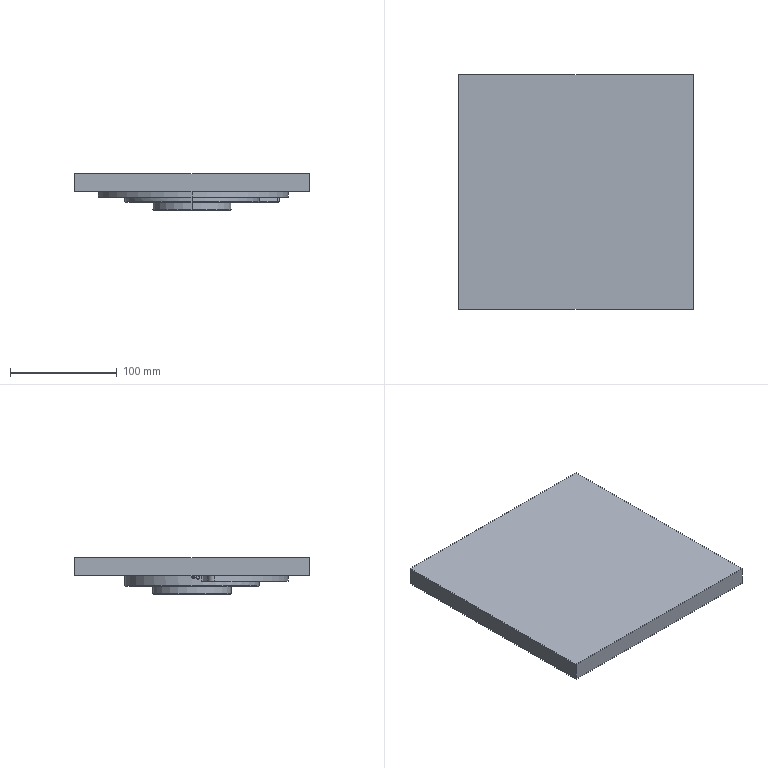NC program | NX | posted with a generic post | part box 220 x 220 x 34.5 mm
Lines 4490 to 5339 of 14163:
(ZLEVEL_PROFILE_COPY_1_COPY , TOOL : D4)
N8918 T10 M6
N8920 G54
N8922 G17 G0 G90 X68.105 Y9.166 S9500 M3
N8924 G43 Z30. H10
N8926 Z-0.4
N8928 G94 G1 X67.66 Y9.696 F1000.
N8930 G3 X67.284 Y9.833 R0.4
N8932 G1 X64.343 Y9.315 F1500.
N8934 X64.337 Y9.257
N8936 G2 X64.684 Y6.399 R65.
N8938 G3 X64.917 Y6.074 R0.4
N8940 G1 X65.545 Y5.79
N8942 G0 X68.105 Y9.166 Z-0.8
N8944 G1 X67.66 Y9.696 F1000.
N8946 G3 X67.284 Y9.833 R0.4
N8948 G1 X64.343 Y9.315 F1500.
N8950 X64.337 Y9.257
N8952 G2 X64.684 Y6.398 R65.
N8954 G3 X64.917 Y6.073 R0.4
N8956 G1 X65.545 Y5.789
N8958 G0 X68.105 Y9.166 Z-1.2
N8960 G1 X67.66 Y9.696 F1000.
N8962 G3 X67.284 Y9.833 R0.4
N8964 G1 X64.343 Y9.315 F1500.
N8966 X64.337 Y9.257
N8968 G2 X64.684 Y6.397 R65.
N8970 G3 X64.918 Y6.072 R0.4
N8972 G1 X65.545 Y5.788
N8974 G0 X68.105 Y9.166 Z-1.6
N8976 G1 X67.66 Y9.696 F1000.
N8978 G3 X67.284 Y9.833 R0.4
N8980 G1 X64.343 Y9.315 F1500.
N8982 X64.338 Y9.257
N8984 G2 X64.685 Y6.396 R65.
N8986 G3 X64.918 Y6.071 R0.4
N8988 G1 X65.545 Y5.787
N8990 G0 X68.105 Y9.166 Z-2.
N8992 G1 X67.66 Y9.696 F1000.
N8994 G3 X67.284 Y9.833 R0.4
N8996 G1 X64.343 Y9.315 F1500.
N8998 X64.338 Y9.257
N9000 G2 X64.685 Y6.395 R65.
N9002 G3 X64.918 Y6.069 R0.4
N9004 G1 X65.545 Y5.786
N9006 G0 X68.105 Y9.166 Z-2.4
N9008 G1 X67.66 Y9.696 F1000.
N9010 G3 X67.284 Y9.833 R0.4
N9012 G1 X64.343 Y9.315 F1500.
N9014 X64.338 Y9.256
N9016 G2 X64.685 Y6.393 R65.
N9018 G3 X64.918 Y6.068 R0.4
N9020 G1 X65.545 Y5.784
N9022 G0 X68.105 Y9.166 Z-2.8
N9024 G1 X67.66 Y9.696 F1000.
N9026 G3 X67.284 Y9.833 R0.4
N9028 G1 X64.343 Y9.315 F1500.
N9030 X64.338 Y9.256
N9032 G2 X64.686 Y6.386 R65.
N9034 G3 X64.919 Y6.061 R0.4
N9036 G1 X65.546 Y5.777
N9038 G0 X68.105 Y9.166 Z-3.2
N9040 G1 X67.66 Y9.696 F1000.
N9042 G3 X67.284 Y9.833 R0.4
N9044 G1 X64.343 Y9.315 F1500.
N9046 X64.338 Y9.256
N9048 G2 X64.686 Y6.386 R65.
N9050 G3 X64.919 Y6.061 R0.4
N9052 G1 X65.546 Y5.777
N9054 G0 X68.105 Y9.166 Z-3.6
N9056 G1 X67.66 Y9.696 F1000.
N9058 G3 X67.284 Y9.833 R0.4
N9060 G1 X64.343 Y9.315 F1500.
N9062 X64.338 Y9.256
N9064 G2 X64.686 Y6.386 R65.
N9066 G3 X64.919 Y6.061 R0.4
N9068 G1 X65.546 Y5.777
N9070 G0 X68.105 Y9.166 Z-4.
N9072 G1 X67.66 Y9.696 F1000.
N9074 G3 X67.284 Y9.833 R0.4
N9076 G1 X64.343 Y9.315 F1500.
N9078 X64.338 Y9.256
N9080 G2 X64.686 Y6.386 R65.
N9082 G3 X64.919 Y6.061 R0.4
N9084 G1 X65.546 Y5.777
N9086 G0 X68.105 Y9.166 Z-4.4
N9088 G1 X67.66 Y9.696 F1000.
N9090 G3 X67.284 Y9.833 R0.4
N9092 G1 X64.343 Y9.315 F1500.
N9094 X64.338 Y9.256
N9096 G2 X64.686 Y6.386 R65.
N9098 G3 X64.919 Y6.061 R0.4
N9100 G1 X65.546 Y5.777
N9102 G0 X68.105 Y9.166 Z-4.8
N9104 G1 X67.66 Y9.696 F1000.
N9106 G3 X67.284 Y9.833 R0.4
N9108 G1 X64.343 Y9.315 F1500.
N9110 X64.338 Y9.256
N9112 G2 X64.686 Y6.386 R65.
N9114 G3 X64.919 Y6.061 R0.4
N9116 G1 X65.546 Y5.777
N9118 G0 X68.105 Y9.166 Z-5.2
N9120 G1 X67.66 Y9.696 F1000.
N9122 G3 X67.284 Y9.833 R0.4
N9124 G1 X64.343 Y9.315 F1500.
N9126 X64.338 Y9.256
N9128 G2 X64.686 Y6.386 R65.
N9130 G3 X64.919 Y6.061 R0.4
N9132 G1 X65.546 Y5.777
N9134 G0 X68.105 Y9.166 Z-5.6
N9136 G1 X67.66 Y9.696 F1000.
N9138 G3 X67.284 Y9.833 R0.4
N9140 G1 X64.343 Y9.315 F1500.
N9142 X64.338 Y9.256
N9144 G2 X64.686 Y6.386 R65.
N9146 G3 X64.919 Y6.061 R0.4
N9148 G1 X65.546 Y5.777
N9150 G0 X68.105 Y9.166 Z-6.
N9152 G1 X67.66 Y9.696 F1000.
N9154 G3 X67.284 Y9.833 R0.4
N9156 G1 X64.343 Y9.315 F1500.
N9158 X64.338 Y9.256
N9160 G2 X64.686 Y6.386 R65.
N9162 G3 X64.919 Y6.061 R0.4
N9164 G1 X65.546 Y5.777
N9166 G0 X68.105 Y9.166 Z-6.4
N9168 G1 X67.66 Y9.696 F1000.
N9170 G3 X67.284 Y9.833 R0.4
N9172 G1 X64.343 Y9.315 F1500.
N9174 X64.338 Y9.256
N9176 G2 X64.686 Y6.386 R65.
N9178 G3 X64.919 Y6.061 R0.4
N9180 G1 X65.546 Y5.777
N9182 G0 X68.105 Y9.166 Z-6.8
N9184 G1 X67.66 Y9.696 F1000.
N9186 G3 X67.284 Y9.833 R0.4
N9188 G1 X64.343 Y9.315 F1500.
N9190 X64.338 Y9.256
N9192 G2 X64.685 Y6.388 R65.
N9194 G3 X64.918 Y6.062 R0.4
N9196 G1 X65.545 Y5.779
N9198 G0 X68.105 Y9.166 Z-7.2
N9200 G1 X67.659 Y9.696 F1000.
N9202 G3 X67.284 Y9.833 R0.4
N9204 G1 X64.343 Y9.315 F1500.
N9206 X64.338 Y9.255
N9208 G2 X64.523 Y7.856 R65.
N9210 G1 X64.651 Y6.699
N9212 G3 X64.888 Y6.377 R0.4
N9214 G1 X65.517 Y6.101
N9216 G0 X68.105 Y9.166 Z-7.6
N9218 G1 X67.66 Y9.696 F1000.
N9220 G3 X67.284 Y9.833 R0.4
N9222 G1 X64.343 Y9.315 F1500.
N9224 X64.338 Y9.255
N9226 G2 X64.523 Y7.856 R65.
N9228 G1 X64.522 Y7.838
N9230 X64.598 Y7.19
N9232 X64.613 Y7.053
N9234 X64.651 Y6.699
N9236 G3 X64.886 Y6.376 R0.4
N9238 G1 X65.517 Y6.096
N9240 G0 X68.105 Y9.166 Z-8.
N9242 G1 X67.66 Y9.696 F1000.
N9244 G3 X67.284 Y9.833 R0.4
N9246 G1 X64.343 Y9.315 F1500.
N9248 X64.338 Y9.255
N9250 G2 X64.523 Y7.856 R65.
N9252 G1 X64.522 Y7.838
N9254 X64.599 Y7.19
N9256 X64.613 Y7.053
N9258 X64.651 Y6.699
N9260 G3 X64.886 Y6.376 R0.4
N9262 G1 X65.517 Y6.096
N9264 G0 X68.105 Y9.166 Z-8.4
N9266 G1 X67.66 Y9.696 F1000.
N9268 G3 X67.284 Y9.833 R0.4
N9270 G1 X64.343 Y9.315 F1500.
N9272 X64.338 Y9.255
N9274 G2 X64.523 Y7.856 R65.
N9276 G1 X64.522 Y7.838
N9278 X64.599 Y7.19
N9280 X64.613 Y7.053
N9282 X64.651 Y6.699
N9284 G3 X64.886 Y6.376 R0.4
N9286 G1 X65.517 Y6.096
N9288 G0 X68.105 Y9.166 Z-8.8
N9290 G1 X67.66 Y9.696 F1000.
N9292 G3 X67.284 Y9.833 R0.4
N9294 G1 X64.343 Y9.315 F1500.
N9296 X64.338 Y9.255
N9298 G2 X64.523 Y7.856 R65.
N9300 G1 X64.522 Y7.838
N9302 X64.613 Y7.062
N9304 X64.651 Y6.699
N9306 G3 X64.887 Y6.376 R0.4
N9308 G1 X65.517 Y6.097
N9310 G0 X68.106 Y9.166 Z-9.2
N9312 G1 X67.66 Y9.696 F1000.
N9314 G3 X67.284 Y9.833 R0.4
N9316 G1 X64.343 Y9.315 F1500.
N9318 X64.338 Y9.255
N9320 G2 X64.523 Y7.856 R65.
N9322 G1 X64.629 Y6.908
N9324 X64.651 Y6.699
N9326 G3 X64.885 Y6.375 R0.4
N9328 G1 X65.518 Y6.089
N9330 G0 X68.106 Y9.166 Z-9.6
N9332 G1 X67.66 Y9.696 F1000.
N9334 G3 X67.284 Y9.833 R0.4
N9336 G1 X64.343 Y9.315 F1500.
N9338 X64.338 Y9.255
N9340 G2 X64.523 Y7.856 R65.
N9342 G3 X64.764 Y7.537 R0.4
N9344 G1 X65.391 Y7.269
N9346 G0 X68.106 Y9.166 Z-10.
N9348 G1 X67.66 Y9.696 F1000.
N9350 G3 X67.285 Y9.833 R0.4
N9352 G1 X64.343 Y9.315 F1500.
N9354 X64.338 Y9.255
N9356 G2 X64.523 Y7.856 R65.
N9358 G3 X64.764 Y7.537 R0.4
N9360 G1 X65.391 Y7.27
N9362 G0 X68.106 Y9.166 Z-10.4
N9364 G1 X67.66 Y9.696 F1000.
N9366 G3 X67.285 Y9.833 R0.4
N9368 G1 X64.343 Y9.315 F1500.
N9370 X64.338 Y9.255
N9372 G2 X64.523 Y7.856 R65.
N9374 G3 X64.764 Y7.537 R0.4
N9376 G1 X65.391 Y7.269
N9378 G0 X68.106 Y9.166 Z-10.8
N9380 G1 X67.66 Y9.696 F1000.
N9382 G3 X67.285 Y9.833 R0.4
N9384 G1 X64.343 Y9.315 F1500.
N9386 X64.338 Y9.255
N9388 G2 X64.523 Y7.856 R65.
N9390 G3 X64.764 Y7.537 R0.4
N9392 G1 X65.391 Y7.269
N9394 G0 X68.106 Y9.166 Z-11.2
N9396 G1 X67.66 Y9.696 F1000.
N9398 G3 X67.285 Y9.833 R0.4
N9400 G1 X64.343 Y9.315 F1500.
N9402 X64.338 Y9.255
N9404 G2 X64.523 Y7.856 R65.
N9406 G3 X64.764 Y7.537 R0.4
N9408 G1 X65.391 Y7.269
N9410 G0 X68.106 Y9.166 Z-11.6
N9412 G1 X67.66 Y9.696 F1000.
N9414 G3 X67.285 Y9.833 R0.4
N9416 G1 X64.343 Y9.315 F1500.
N9418 X64.338 Y9.254
N9420 G2 X64.523 Y7.856 R65.
N9422 G3 X64.764 Y7.537 R0.4
N9424 G1 X65.391 Y7.269
N9426 G0 X68.106 Y9.166 Z-12.
N9428 G1 X67.66 Y9.696 F1000.
N9430 G3 X67.285 Y9.833 R0.4
N9432 G1 X64.343 Y9.315 F1500.
N9434 X64.338 Y9.254
N9436 G2 X64.523 Y7.856 R65.
N9438 G3 X64.764 Y7.537 R0.4
N9440 G1 X65.391 Y7.269
N9442 G0 X68.106 Y9.166 Z-12.385
N9444 G1 X67.66 Y9.696 F1000.
N9446 G3 X67.285 Y9.833 R0.4
N9448 G1 X64.343 Y9.315 F1500.
N9450 X64.338 Y9.254
N9452 G2 X64.523 Y7.856 R65.
N9454 G3 X64.764 Y7.537 R0.4
N9456 G1 X65.391 Y7.269
N9458 G0 X68.106 Y9.166 Z-12.769
N9460 G1 X67.66 Y9.696 F1000.
N9462 G3 X67.285 Y9.833 R0.4
N9464 G1 X64.343 Y9.315 F1500.
N9466 X64.338 Y9.254
N9468 G2 X64.523 Y7.856 R65.
N9470 G3 X64.764 Y7.537 R0.4
N9472 G1 X65.391 Y7.269
N9474 G0 X65.242 Y8.555 Z-13.154
N9476 G1 X64.719 Y9.178 F1000.
N9478 G3 X64.343 Y9.315 R0.4
N9480 G1 X64.338 Y9.254 F1500.
N9482 G2 X64.523 Y7.856 R65.
N9484 G3 X64.764 Y7.537 R0.4
N9486 G1 X65.391 Y7.269
N9488 G0 X65.242 Y8.555 Z-13.538
N9490 G1 X64.719 Y9.178 F1000.
N9492 G3 X64.343 Y9.315 R0.4
N9494 G1 X64.338 Y9.254 F1500.
N9496 G2 X64.523 Y7.856 R65.
N9498 G3 X64.764 Y7.537 R0.4
N9500 G1 X65.391 Y7.269
N9502 G0 X65.242 Y8.555 Z-13.923
N9504 G1 X64.719 Y9.178 F1000.
N9506 G3 X64.343 Y9.315 R0.4
N9508 G1 X64.338 Y9.254 F1500.
N9510 G2 X64.523 Y7.856 R65.
N9512 G3 X64.764 Y7.537 R0.4
N9514 G1 X65.391 Y7.269
N9516 G0 X65.242 Y8.555 Z-14.308
N9518 G1 X64.719 Y9.178 F1000.
N9520 G3 X64.343 Y9.315 R0.4
N9522 G1 X64.338 Y9.254 F1500.
N9524 G2 X64.523 Y7.856 R65.
N9526 G3 X64.764 Y7.537 R0.4
N9528 G1 X65.391 Y7.269
N9530 G0 X65.242 Y8.555 Z-14.692
N9532 G1 X64.719 Y9.178 F1000.
N9534 G3 X64.343 Y9.315 R0.4
N9536 G1 X64.338 Y9.254 F1500.
N9538 G2 X64.523 Y7.856 R65.
N9540 G3 X64.764 Y7.537 R0.4
N9542 G1 X65.391 Y7.269
N9544 G0 X65.242 Y8.555 Z-15.077
N9546 G1 X64.719 Y9.178 F1000.
N9548 G3 X64.343 Y9.315 R0.4
N9550 G1 X64.338 Y9.254 F1500.
N9552 G2 X64.523 Y7.856 R65.
N9554 G3 X64.764 Y7.537 R0.4
N9556 G1 X65.391 Y7.269
N9558 G0 X65.242 Y8.555 Z-15.462
N9560 G1 X64.719 Y9.178 F1000.
N9562 G3 X64.343 Y9.315 R0.4
N9564 G1 X64.338 Y9.254 F1500.
N9566 G2 X64.523 Y7.856 R65.
N9568 G3 X64.764 Y7.537 R0.4
N9570 G1 X65.391 Y7.269
N9572 G0 X65.242 Y8.555 Z-15.846
N9574 G1 X64.719 Y9.178 F1000.
N9576 G3 X64.343 Y9.315 R0.4
N9578 G1 X64.338 Y9.254 F1500.
N9580 G2 X64.523 Y7.856 R65.
N9582 G3 X64.764 Y7.537 R0.4
N9584 G1 X65.391 Y7.269
N9586 G0 X65.242 Y8.555 Z-16.231
N9588 G1 X64.719 Y9.178 F1000.
N9590 G3 X64.343 Y9.315 R0.4
N9592 G1 X64.338 Y9.254 F1500.
N9594 G2 X64.523 Y7.856 R65.
N9596 G3 X64.764 Y7.537 R0.4
N9598 G1 X65.391 Y7.269
N9600 G0 X65.228 Y8.658 Z-16.615
N9602 G1 X64.361 Y9.283 F1000.
N9604 X64.338 Y9.234
N9606 X64.348 Y9.18
N9608 G2 X64.523 Y7.856 R65. F1500.
N9610 G3 X64.764 Y7.537 R0.4
N9612 G1 X65.391 Y7.269
N9614 G0 X65.228 Y8.658 Z-17.
N9616 G1 X64.361 Y9.283 F1000.
N9618 X64.338 Y9.234
N9620 X64.348 Y9.18
N9622 G2 X64.523 Y7.856 R65. F1500.
N9624 G3 X64.764 Y7.537 R0.4
N9626 G1 X65.391 Y7.269
N9628 G0 Z30.
N9630 X-53.927 Y-37.704
N9632 Z-0.4
N9634 G1 X-53.629 Y-37.083 F1000.
N9636 G3 X-53.659 Y-36.684 R0.4
N9638 G2 X-55.245 Y-34.248 R65. F1500.
N9640 G1 X-55.254 Y-34.226
N9642 X-55.277 Y-34.22
N9644 X-55.296 Y-34.234
N9646 X-57.863 Y-35.717
N9648 G3 X-58.063 Y-36.063 R0.4
N9650 G1 Y-36.756
N9652 G0 X-53.927 Y-37.704 Z-0.8
N9654 G1 X-53.629 Y-37.083 F1000.
N9656 G3 X-53.659 Y-36.684 R0.4
N9658 G2 X-55.245 Y-34.248 R65. F1500.
N9660 G1 X-55.254 Y-34.226
N9662 X-55.277 Y-34.22
N9664 X-55.296 Y-34.234
N9666 X-57.863 Y-35.717
N9668 G3 X-58.063 Y-36.063 R0.4
N9670 G1 Y-36.756
N9672 G0 X-53.927 Y-37.704 Z-1.2
N9674 G1 X-53.629 Y-37.083 F1000.
N9676 G3 X-53.659 Y-36.684 R0.4
N9678 G2 X-55.245 Y-34.248 R65. F1500.
N9680 G1 X-55.254 Y-34.226
N9682 X-55.277 Y-34.22
N9684 X-55.296 Y-34.234
N9686 X-57.863 Y-35.717
N9688 G3 X-58.063 Y-36.063 R0.4
N9690 G1 Y-36.756
N9692 G0 X-53.927 Y-37.704 Z-1.6
N9694 G1 X-53.629 Y-37.083 F1000.
N9696 G3 X-53.659 Y-36.684 R0.4
N9698 G2 X-55.245 Y-34.248 R65. F1500.
N9700 G1 X-55.254 Y-34.226
N9702 X-55.277 Y-34.22
N9704 X-55.296 Y-34.234
N9706 X-57.863 Y-35.717
N9708 G3 X-58.063 Y-36.063 R0.4
N9710 G1 Y-36.756
N9712 G0 X-53.927 Y-37.704 Z-2.
N9714 G1 X-53.629 Y-37.083 F1000.
N9716 G3 X-53.659 Y-36.684 R0.4
N9718 G2 X-55.245 Y-34.248 R65. F1500.
N9720 G1 X-55.254 Y-34.226
N9722 X-55.277 Y-34.22
N9724 X-55.296 Y-34.234
N9726 X-57.863 Y-35.717
N9728 G3 X-58.063 Y-36.063 R0.4
N9730 G1 Y-36.756
N9732 G0 X-53.927 Y-37.704 Z-2.4
N9734 G1 X-53.629 Y-37.083 F1000.
N9736 G3 X-53.659 Y-36.684 R0.4
N9738 G2 X-55.245 Y-34.248 R65. F1500.
N9740 G1 X-55.254 Y-34.226
N9742 X-55.277 Y-34.22
N9744 X-55.296 Y-34.234
N9746 X-57.863 Y-35.717
N9748 G3 X-58.063 Y-36.063 R0.4
N9750 G1 Y-36.756
N9752 G0 X-53.927 Y-37.704 Z-2.8
N9754 G1 X-53.629 Y-37.083 F1000.
N9756 G3 X-53.659 Y-36.684 R0.4
N9758 G2 X-55.245 Y-34.248 R65. F1500.
N9760 G1 X-55.254 Y-34.226
N9762 X-55.277 Y-34.22
N9764 X-55.296 Y-34.234
N9766 X-57.863 Y-35.717
N9768 G3 X-58.063 Y-36.063 R0.4
N9770 G1 Y-36.756
N9772 G0 X-53.927 Y-37.704 Z-3.2
N9774 G1 X-53.629 Y-37.083 F1000.
N9776 G3 X-53.659 Y-36.684 R0.4
N9778 G2 X-55.245 Y-34.248 R65. F1500.
N9780 G1 X-55.254 Y-34.226
N9782 X-55.277 Y-34.22
N9784 X-55.296 Y-34.234
N9786 X-57.863 Y-35.717
N9788 G3 X-58.063 Y-36.063 R0.4
N9790 G1 Y-36.756
N9792 G0 X-53.927 Y-37.704 Z-3.6
N9794 G1 X-53.629 Y-37.083 F1000.
N9796 G3 X-53.659 Y-36.684 R0.4
N9798 G2 X-55.245 Y-34.248 R65. F1500.
N9800 G1 X-55.254 Y-34.226
N9802 X-55.277 Y-34.22
N9804 X-55.296 Y-34.234
N9806 X-57.863 Y-35.717
N9808 G3 X-58.063 Y-36.063 R0.4
N9810 G1 Y-36.756
N9812 G0 X-53.927 Y-37.704 Z-4.
N9814 G1 X-53.629 Y-37.083 F1000.
N9816 G3 X-53.659 Y-36.684 R0.4
N9818 G2 X-55.245 Y-34.248 R65. F1500.
N9820 G1 X-55.254 Y-34.226
N9822 X-55.277 Y-34.22
N9824 X-55.296 Y-34.234
N9826 X-57.863 Y-35.717
N9828 G3 X-58.063 Y-36.063 R0.4
N9830 G1 Y-36.756
N9832 G0 X-53.927 Y-37.704 Z-4.4
N9834 G1 X-53.629 Y-37.083 F1000.
N9836 G3 X-53.659 Y-36.684 R0.4
N9838 G2 X-55.245 Y-34.248 R65. F1500.
N9840 G1 X-55.254 Y-34.226
N9842 X-55.277 Y-34.22
N9844 X-55.296 Y-34.234
N9846 X-57.863 Y-35.717
N9848 G3 X-58.063 Y-36.063 R0.4
N9850 G1 Y-36.756
N9852 G0 X-53.927 Y-37.704 Z-4.8
N9854 G1 X-53.629 Y-37.083 F1000.
N9856 G3 X-53.659 Y-36.684 R0.4
N9858 G2 X-55.245 Y-34.248 R65. F1500.
N9860 G1 X-55.254 Y-34.226
N9862 X-55.277 Y-34.22
N9864 X-55.296 Y-34.234
N9866 X-57.863 Y-35.717
N9868 G3 X-58.063 Y-36.063 R0.4
N9870 G1 Y-36.756
N9872 G0 X-53.927 Y-37.704 Z-5.2
N9874 G1 X-53.629 Y-37.083 F1000.
N9876 G3 X-53.659 Y-36.684 R0.4
N9878 G2 X-55.245 Y-34.248 R65. F1500.
N9880 G1 X-55.254 Y-34.226
N9882 X-55.277 Y-34.22
N9884 X-55.296 Y-34.234
N9886 X-57.863 Y-35.717
N9888 G3 X-58.063 Y-36.063 R0.4
N9890 G1 Y-36.756
N9892 G0 X-53.927 Y-37.704 Z-5.6
N9894 G1 X-53.629 Y-37.083 F1000.
N9896 G3 X-53.659 Y-36.684 R0.4
N9898 G2 X-55.245 Y-34.248 R65. F1500.
N9900 G1 X-55.254 Y-34.226
N9902 X-55.277 Y-34.22
N9904 X-55.296 Y-34.234
N9906 X-57.863 Y-35.717
N9908 G3 X-58.063 Y-36.063 R0.4
N9910 G1 Y-36.756
N9912 G0 X-53.927 Y-37.704 Z-6.
N9914 G1 X-53.629 Y-37.083 F1000.
N9916 G3 X-53.659 Y-36.684 R0.4
N9918 G2 X-55.245 Y-34.248 R65. F1500.
N9920 G1 X-55.254 Y-34.226
N9922 X-55.277 Y-34.22
N9924 X-55.296 Y-34.234
N9926 X-57.863 Y-35.717
N9928 G3 X-58.063 Y-36.063 R0.4
N9930 G1 Y-36.756
N9932 G0 X-53.927 Y-37.704 Z-6.4
N9934 G1 X-53.629 Y-37.083 F1000.
N9936 G3 X-53.659 Y-36.684 R0.4
N9938 G2 X-55.245 Y-34.248 R65. F1500.
N9940 G1 X-55.254 Y-34.226
N9942 X-55.277 Y-34.22
N9944 X-55.296 Y-34.234
N9946 X-57.863 Y-35.717
N9948 G3 X-58.063 Y-36.063 R0.4
N9950 G1 Y-36.756
N9952 G0 X-53.927 Y-37.704 Z-6.8
N9954 G1 X-53.629 Y-37.083 F1000.
N9956 G3 X-53.659 Y-36.684 R0.4
N9958 G2 X-55.245 Y-34.248 R65. F1500.
N9960 G1 X-55.254 Y-34.226
N9962 X-55.277 Y-34.22
N9964 X-55.296 Y-34.234
N9966 X-57.863 Y-35.717
N9968 G3 X-58.063 Y-36.063 R0.4
N9970 G1 Y-36.756
N9972 G0 X-53.927 Y-37.704 Z-7.2
N9974 G1 X-53.629 Y-37.083 F1000.
N9976 G3 X-53.659 Y-36.684 R0.4
N9978 G2 X-55.245 Y-34.248 R65. F1500.
N9980 G1 X-55.254 Y-34.226
N9982 X-55.277 Y-34.22
N9984 X-55.296 Y-34.234
N9986 X-57.863 Y-35.717
N9988 G3 X-58.063 Y-36.063 R0.4
N9990 G1 Y-36.756
N9992 G0 X-53.927 Y-37.704 Z-7.6
N9994 G1 X-53.629 Y-37.083 F1000.
N9996 G3 X-53.659 Y-36.684 R0.4
N9998 G2 X-55.245 Y-34.248 R65. F1500.
N10000 G1 X-55.254 Y-34.226
N10002 X-55.277 Y-34.22
N10004 X-55.296 Y-34.234
N10006 X-57.863 Y-35.717
N10008 G3 X-58.063 Y-36.063 R0.4
N10010 G1 Y-36.756
N10012 G0 X-53.927 Y-37.704 Z-8.
N10014 G1 X-53.629 Y-37.083 F1000.
N10016 G3 X-53.659 Y-36.684 R0.4
N10018 G2 X-55.245 Y-34.248 R65. F1500.
N10020 G1 X-55.254 Y-34.226
N10022 X-55.277 Y-34.22
N10024 X-55.296 Y-34.234
N10026 X-57.863 Y-35.717
N10028 G3 X-58.063 Y-36.063 R0.4
N10030 G1 Y-36.756
N10032 G0 X-53.927 Y-37.704 Z-8.4
N10034 G1 X-53.629 Y-37.083 F1000.
N10036 G3 X-53.659 Y-36.684 R0.4
N10038 G2 X-55.245 Y-34.248 R65. F1500.
N10040 G1 X-55.254 Y-34.226
N10042 X-55.277 Y-34.22
N10044 X-55.296 Y-34.234
N10046 X-57.863 Y-35.717
N10048 G3 X-58.063 Y-36.063 R0.4
N10050 G1 Y-36.756
N10052 G0 X-53.927 Y-37.704 Z-8.8
N10054 G1 X-53.629 Y-37.083 F1000.
N10056 G3 X-53.659 Y-36.684 R0.4
N10058 G2 X-55.245 Y-34.248 R65. F1500.
N10060 G1 X-55.254 Y-34.226
N10062 X-55.277 Y-34.22
N10064 X-55.296 Y-34.234
N10066 X-57.863 Y-35.717
N10068 G3 X-58.063 Y-36.063 R0.4
N10070 G1 Y-36.756
N10072 G0 X-53.927 Y-37.704 Z-9.2
N10074 G1 X-53.629 Y-37.083 F1000.
N10076 G3 X-53.659 Y-36.684 R0.4
N10078 G2 X-55.245 Y-34.248 R65. F1500.
N10080 G1 X-55.254 Y-34.226
N10082 X-55.277 Y-34.22
N10084 X-55.296 Y-34.234
N10086 X-57.863 Y-35.717
N10088 G3 X-58.063 Y-36.063 R0.4
N10090 G1 Y-36.756
N10092 G0 X-53.927 Y-37.704 Z-9.6
N10094 G1 X-53.629 Y-37.083 F1000.
N10096 G3 X-53.659 Y-36.684 R0.4
N10098 G2 X-55.245 Y-34.248 R65. F1500.
N10100 G1 X-55.254 Y-34.226
N10102 X-55.277 Y-34.22
N10104 X-55.296 Y-34.234
N10106 X-57.863 Y-35.717
N10108 G3 X-58.063 Y-36.063 R0.4
N10110 G1 Y-36.756
N10112 G0 X-53.927 Y-37.704 Z-10.
N10114 G1 X-53.629 Y-37.083 F1000.
N10116 G3 X-53.659 Y-36.684 R0.4
N10118 G2 X-55.245 Y-34.248 R65. F1500.
N10120 G1 X-55.254 Y-34.226
N10122 X-55.277 Y-34.22
N10124 X-55.296 Y-34.234
N10126 X-57.863 Y-35.717
N10128 G3 X-58.063 Y-36.063 R0.4
N10130 G1 Y-36.756
N10132 G0 X-53.927 Y-37.704 Z-10.4
N10134 G1 X-53.629 Y-37.083 F1000.
N10136 G3 X-53.659 Y-36.684 R0.4
N10138 G2 X-55.245 Y-34.248 R65. F1500.
N10140 G1 X-55.254 Y-34.226
N10142 X-55.277 Y-34.22
N10144 X-55.296 Y-34.234
N10146 X-57.863 Y-35.717
N10148 G3 X-58.063 Y-36.063 R0.4
N10150 G1 Y-36.756
N10152 G0 X-53.927 Y-37.704 Z-10.8
N10154 G1 X-53.629 Y-37.083 F1000.
N10156 G3 X-53.659 Y-36.684 R0.4
N10158 G2 X-55.245 Y-34.248 R65. F1500.
N10160 G1 X-55.254 Y-34.226
N10162 X-55.277 Y-34.22
N10164 X-55.296 Y-34.234
N10166 X-57.863 Y-35.717
N10168 G3 X-58.063 Y-36.063 R0.4
N10170 G1 Y-36.756
N10172 G0 X-53.927 Y-37.704 Z-11.2
N10174 G1 X-53.629 Y-37.083 F1000.
N10176 G3 X-53.659 Y-36.684 R0.4
N10178 G2 X-55.245 Y-34.248 R65. F1500.
N10180 G1 X-55.254 Y-34.226
N10182 X-55.277 Y-34.22
N10184 X-55.296 Y-34.234
N10186 X-57.863 Y-35.717
N10188 G3 X-58.063 Y-36.063 R0.4
N10190 G1 Y-36.756
N10192 G0 X-53.927 Y-37.704 Z-11.6
N10194 G1 X-53.629 Y-37.083 F1000.
N10196 G3 X-53.659 Y-36.684 R0.4
N10198 G2 X-55.245 Y-34.248 R65. F1500.
N10200 G1 X-55.254 Y-34.226
N10202 X-55.277 Y-34.22
N10204 X-55.296 Y-34.234
N10206 X-57.863 Y-35.717
N10208 G3 X-58.063 Y-36.063 R0.4
N10210 G1 Y-36.756
N10212 G0 X-53.927 Y-37.704 Z-12.
N10214 G1 X-53.629 Y-37.083 F1000.
N10216 G3 X-53.659 Y-36.684 R0.4
N10218 G2 X-55.245 Y-34.248 R65. F1500.
N10220 G1 X-55.254 Y-34.226
N10222 X-55.277 Y-34.22
N10224 X-55.296 Y-34.234
N10226 X-57.863 Y-35.717
N10228 G3 X-58.063 Y-36.063 R0.4
N10230 G1 Y-36.756
N10232 G0 X-53.927 Y-37.704 Z-12.385
N10234 G1 X-53.629 Y-37.083 F1000.
N10236 G3 X-53.659 Y-36.684 R0.4
N10238 G2 X-55.245 Y-34.248 R65. F1500.
N10240 G1 X-55.254 Y-34.226
N10242 X-55.277 Y-34.22
N10244 X-55.296 Y-34.234
N10246 X-57.863 Y-35.717
N10248 G3 X-58.063 Y-36.063 R0.4
N10250 G1 Y-36.756
N10252 G0 X-53.927 Y-37.704 Z-12.769
N10254 G1 X-53.629 Y-37.083 F1000.
N10256 G3 X-53.659 Y-36.684 R0.4
N10258 G2 X-55.245 Y-34.248 R65. F1500.
N10260 G1 X-55.254 Y-34.226
N10262 X-55.277 Y-34.22
N10264 X-55.296 Y-34.234
N10266 X-57.863 Y-35.717
N10268 G3 X-58.063 Y-36.063 R0.4
N10270 G1 Y-36.756
N10272 G0 X-53.927 Y-37.704 Z-13.154
N10274 G1 X-53.629 Y-37.083 F1000.
N10276 G3 X-53.659 Y-36.684 R0.4
N10278 G2 X-55.245 Y-34.248 R65. F1500.
N10280 G1 X-55.254 Y-34.226
N10282 X-55.277 Y-34.22
N10284 X-55.296 Y-34.234
N10286 X-57.863 Y-35.717
N10288 G3 X-58.063 Y-36.063 R0.4
N10290 G1 Y-36.756
N10292 G0 X-53.927 Y-37.704 Z-13.538
N10294 G1 X-53.629 Y-37.083 F1000.
N10296 G3 X-53.659 Y-36.684 R0.4
N10298 G2 X-55.245 Y-34.248 R65. F1500.
N10300 G1 X-55.254 Y-34.226
N10302 X-55.277 Y-34.22
N10304 X-55.296 Y-34.234
N10306 X-57.863 Y-35.717
N10308 G3 X-58.063 Y-36.063 R0.4
N10310 G1 Y-36.756
N10312 G0 X-53.927 Y-37.704 Z-13.923
N10314 G1 X-53.629 Y-37.083 F1000.
N10316 G3 X-53.659 Y-36.684 R0.4
N10318 G2 X-55.245 Y-34.248 R65. F1500.
N10320 G1 X-55.254 Y-34.226
N10322 X-55.277 Y-34.22
N10324 X-55.296 Y-34.234
N10326 X-57.863 Y-35.717
N10328 G3 X-58.063 Y-36.063 R0.4
N10330 G1 Y-36.756
N10332 G0 X-53.927 Y-37.704 Z-14.308
N10334 G1 X-53.629 Y-37.083 F1000.
N10336 G3 X-53.659 Y-36.684 R0.4
N10338 G2 X-55.245 Y-34.248 R65. F1500.
N10340 G1 X-55.254 Y-34.226
N10342 X-55.277 Y-34.22
N10344 X-55.296 Y-34.234
N10346 X-57.863 Y-35.717
N10348 G3 X-58.063 Y-36.063 R0.4
N10350 G1 Y-36.756
N10352 G0 X-53.927 Y-37.704 Z-14.692
N10354 G1 X-53.629 Y-37.083 F1000.
N10356 G3 X-53.659 Y-36.684 R0.4
N10358 G2 X-55.245 Y-34.248 R65. F1500.
N10360 G1 X-55.254 Y-34.226
N10362 X-55.277 Y-34.22
N10364 X-55.296 Y-34.234
N10366 X-57.863 Y-35.717
N10368 G3 X-58.063 Y-36.063 R0.4
N10370 G1 Y-36.756
N10372 G0 X-53.927 Y-37.704 Z-15.077
N10374 G1 X-53.629 Y-37.083 F1000.
N10376 G3 X-53.659 Y-36.684 R0.4
N10378 G2 X-55.239 Y-34.258 R65. F1500.
N10380 G1 X-55.247 Y-34.233
N10382 X-55.272 Y-34.223
N10384 X-55.296 Y-34.234
N10386 X-57.863 Y-35.717
N10388 G3 X-58.063 Y-36.063 R0.4
N10390 G1 Y-36.756
N10392 G0 X-53.927 Y-37.704 Z-15.462
N10394 G1 X-53.629 Y-37.083 F1000.
N10396 G3 X-53.659 Y-36.684 R0.4
N10398 G2 X-55.239 Y-34.258 R65. F1500.
N10400 G1 X-55.247 Y-34.233
N10402 X-55.272 Y-34.223
N10404 X-55.296 Y-34.234
N10406 X-57.863 Y-35.717
N10408 G3 X-58.063 Y-36.063 R0.4
N10410 G1 Y-36.756
N10412 G0 X-53.927 Y-37.704 Z-15.846
N10414 G1 X-53.629 Y-37.083 F1000.
N10416 G3 X-53.659 Y-36.684 R0.4
N10418 G2 X-55.239 Y-34.258 R65. F1500.
N10420 G1 X-55.247 Y-34.233
N10422 X-55.272 Y-34.223
N10424 X-55.296 Y-34.234
N10426 X-57.863 Y-35.717
N10428 G3 X-58.063 Y-36.063 R0.4
N10430 G1 Y-36.756
N10432 G0 X-53.927 Y-37.704 Z-16.231
N10434 G1 X-53.629 Y-37.083 F1000.
N10436 G3 X-53.659 Y-36.684 R0.4
N10438 G2 X-55.239 Y-34.258 R65. F1500.
N10440 G1 X-55.248 Y-34.233
N10442 X-55.272 Y-34.223
N10444 X-55.296 Y-34.234
N10446 X-57.863 Y-35.717
N10448 G3 X-58.063 Y-36.063 R0.4
N10450 G1 Y-36.756
N10452 G0 X-53.927 Y-37.704 Z-16.615
N10454 G1 X-53.629 Y-37.083 F1000.
N10456 G3 X-53.659 Y-36.684 R0.4
N10458 G2 X-55.239 Y-34.258 R65. F1500.
N10460 G1 X-55.248 Y-34.233
N10462 X-55.272 Y-34.223
N10464 X-55.296 Y-34.234
N10466 X-57.863 Y-35.717
N10468 G3 X-58.063 Y-36.063 R0.4
N10470 G1 Y-36.756
N10472 G0 X-53.927 Y-37.704 Z-17.
N10474 G1 X-53.629 Y-37.083 F1000.
N10476 G3 X-53.659 Y-36.684 R0.4
N10478 G2 X-55.239 Y-34.258 R65. F1500.
N10480 G1 X-55.248 Y-34.233
N10482 X-55.272 Y-34.223
N10484 X-55.296 Y-34.234
N10486 X-57.863 Y-35.717
N10488 G3 X-58.063 Y-36.063 R0.4
N10490 G1 Y-36.756
N10492 G0 Z30.
N10494 M5
(ZLEVEL_PROFILE_COPY_1_COPY_COPY_COPY_COPY_2_COPY , TOOL : D6A45)
N10496 T18 M6
N10498 G54
N10500 G17 G0 G90 X38.58 Y37.31 S7000 M3
N10502 G43 Z30. H18
N10504 Z-1.
N10506 G94 G1 X39.741 Y37.98 F1000.
N10508 G3 X40.041 Y38.5 R0.6
N10510 X36. Y42.541 R4.041
N10512 X40.041 Y38.5 R-4.041
N10514 X39.741 Y39.02 R0.6
N10516 G1 X38.58 Y39.69
N10518 G0 Z30.
N10520 X-35.821 Y-15.613
N10522 Z-1.
N10524 G1 X-36.848 Y-14.751
N10526 G3 X-37.439 Y-14.647 R0.6
N10528 G1 X-51.613 Y-19.806
N10530 G3 X-53.888 Y-25.322 R4.041
N10532 X51.652 Y29.619 R-59.541
N10534 X45.828 Y30.919 R4.041
N10536 G1 X39.792 Y26.693
N10538 G3 X39.221 Y23.956 R2.041
N10540 G2 X40.479 Y21.763 R45.959
N10542 X39.151 Y17.694 R2.959
N10544 G1 X35.03 Y15.719
N10546 G3 X34.007 Y13.143 R2.041
N10548 G2 X-13.143 Y-34.007 R36.459
N10550 G3 X-15.719 Y-35.03 R2.041
N10552 G1 X-17.694 Y-39.151
N10554 G2 X-21.763 Y-40.479 R2.959
N10556 X-34.118 Y-30.792 R45.959
N10558 X-33.799 Y-26.524 R2.959
N10560 G1 X-30.268 Y-23.623
N10562 G3 X-29.89 Y-20.876 R2.041
N10564 G2 X-32.458 Y-16.604 R36.459
N10566 G3 X-37.439 Y-14.647 R4.041
N10568 X-37.824 Y-15.106 R0.6
N10570 G1 X-38.005 Y-16.13
N10572 G0 Z30.
N10574 X-55.319 Y-34.431
N10576 Z-1.
N10578 G1 X-55.186 Y-33.315
N10580 G3 X-55.786 Y-33.315 R0.6
N10582 G1 X-73.005 Y-43.257
N10584 G2 X-81.311 Y-40.767 R5.959
N10586 X88.492 Y21.037 R-90.959
N10588 X83.73 Y13.791 R5.959
N10590 G1 X64.149 Y10.338
N10592 G3 X63.299 Y9.163 R1.041
N10594 G2 X-54.38 Y-33.668 R63.959
N10596 G3 X-55.786 Y-33.315 R1.041
N10598 X-56.086 Y-33.834 R0.6
N10600 G1 Y-34.874
N10602 G0 Z30.
N10604 M5